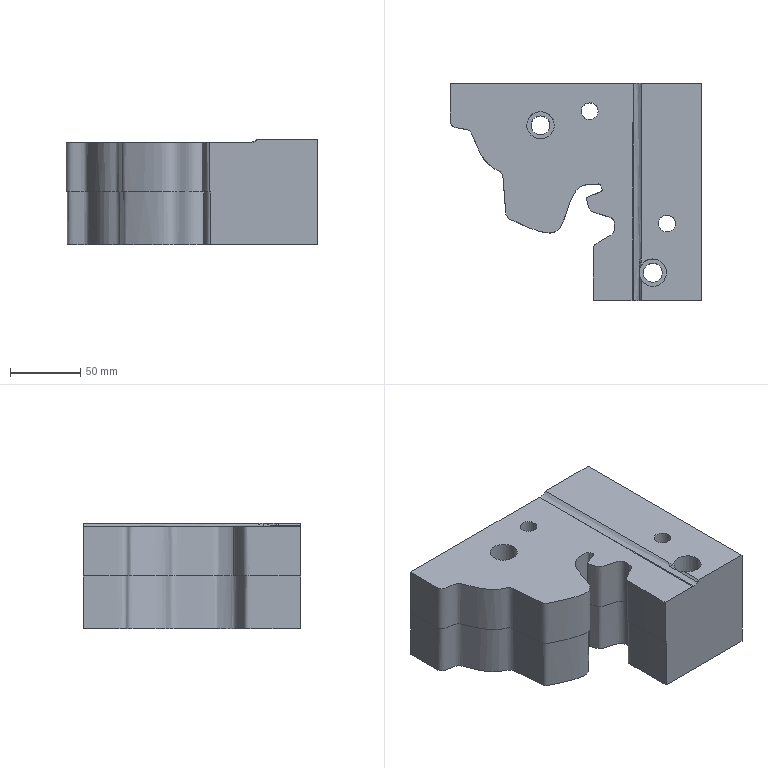Part | NX | features solid 2 | 1 solid | 21 faces | box 179.483 x 155 x 75 mm | volume 1313323 mm3 | spline 8 | plane 7 | cylinder 6 | commonest cylinder face diameters 12 x2 13.5 x2 19.5 x2